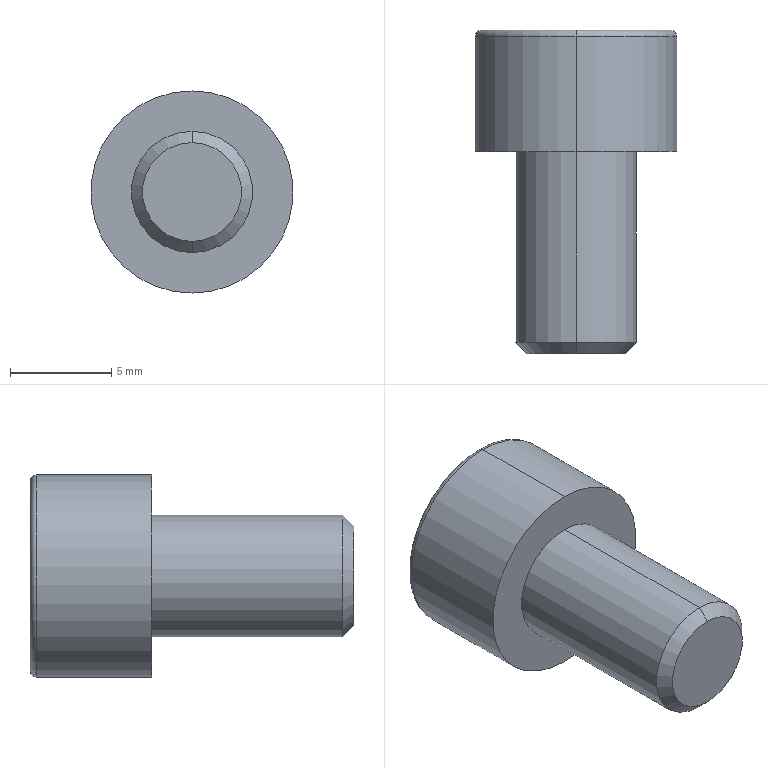Part | SolidWorks | features BaseBody 1 | 1 solid | 18 faces | box 10 x 16 x 10 mm | volume 683.613 mm3 | plane 10 | cylinder 4 | cone 2 | torus 2 | commonest cylinder face diameters 6 x2 10 x2
STEP:
#1=CARTESIAN_POINT('',(0.,-10.,-2.445));
#2=VERTEX_POINT('',#1);
#3=CARTESIAN_POINT('',(0.,-10.,2.445));
#4=VERTEX_POINT('',#3);
#5=CARTESIAN_POINT('',(0.,-10.,0.));
#6=DIRECTION('',(0.,-1.,0.));
#7=DIRECTION('',(0.,0.,-1.));
#8=AXIS2_PLACEMENT_3D('',#5,#6,#7);
#9=CIRCLE('',#8,2.445);
#10=EDGE_CURVE('',#2,#4,#9,.T.);
#11=ORIENTED_EDGE('',*,*,#10,.F.);
#12=CARTESIAN_POINT('',(0.,-9.445,-3.));
#13=VERTEX_POINT('',#12);
#14=CARTESIAN_POINT('',(0.,-10.,-2.445));
#15=DIRECTION('',(0.,0.7071,-0.7071));
#16=VECTOR('',#15,1000.);
#17=LINE('',#14,#16);
#18=EDGE_CURVE('',#2,#13,#17,.T.);
#19=ORIENTED_EDGE('',*,*,#18,.T.);
#20=CARTESIAN_POINT('',(0.,-9.445,3.));
#21=VERTEX_POINT('',#20);
#22=CARTESIAN_POINT('',(0.,-9.445,0.));
#23=DIRECTION('',(0.,1.,0.));
#24=DIRECTION('',(0.,0.,-1.));
#25=AXIS2_PLACEMENT_3D('',#22,#23,#24);
#26=CIRCLE('',#25,3.);
#27=EDGE_CURVE('',#21,#13,#26,.T.);
#28=ORIENTED_EDGE('',*,*,#27,.F.);
#29=CARTESIAN_POINT('',(0.,-10.,2.445));
#30=DIRECTION('',(0.,0.7071,0.7071));
#31=VECTOR('',#30,1000.);
#32=LINE('',#29,#31);
#33=EDGE_CURVE('',#4,#21,#32,.T.);
#34=ORIENTED_EDGE('',*,*,#33,.F.);
#35=EDGE_LOOP('',(#11,#19,#28,#34));
#36=FACE_OUTER_BOUND('',#35,.T.);
#37=CARTESIAN_POINT('',(0.,-10.,0.));
#38=DIRECTION('',(0.,1.,0.));
#39=DIRECTION('',(0.,0.,1.));
#40=AXIS2_PLACEMENT_3D('',#37,#38,#39);
#41=CONICAL_SURFACE('',#40,2.445,0.7854);
#42=ADVANCED_FACE('',(#36),#41,.T.);
#43=ORIENTED_EDGE('',*,*,#27,.T.);
#44=CARTESIAN_POINT('',(0.,0.,-3.));
#45=VERTEX_POINT('',#44);
#46=CARTESIAN_POINT('',(0.,-10.,-3.));
#47=DIRECTION('',(0.,1.,0.));
#48=VECTOR('',#47,1000.);
#49=LINE('',#46,#48);
#50=EDGE_CURVE('',#13,#45,#49,.T.);
#51=ORIENTED_EDGE('',*,*,#50,.T.);
#52=CARTESIAN_POINT('',(0.,0.,3.));
#53=VERTEX_POINT('',#52);
#54=CARTESIAN_POINT('',(0.,0.,0.));
#55=DIRECTION('',(0.,-1.,0.));
#56=DIRECTION('',(0.,0.,1.));
#57=AXIS2_PLACEMENT_3D('',#54,#55,#56);
#58=CIRCLE('',#57,3.);
#59=EDGE_CURVE('',#45,#53,#58,.T.);
#60=ORIENTED_EDGE('',*,*,#59,.T.);
#61=CARTESIAN_POINT('',(0.,-10.,3.));
#62=DIRECTION('',(0.,1.,0.));
#63=VECTOR('',#62,1000.);
#64=LINE('',#61,#63);
#65=EDGE_CURVE('',#21,#53,#64,.T.);
#66=ORIENTED_EDGE('',*,*,#65,.F.);
#67=EDGE_LOOP('',(#43,#51,#60,#66));
#68=FACE_OUTER_BOUND('',#67,.T.);
#69=CARTESIAN_POINT('',(0.,-10.,0.));
#70=DIRECTION('',(0.,1.,0.));
#71=DIRECTION('',(0.,0.,1.));
#72=AXIS2_PLACEMENT_3D('',#69,#70,#71);
#73=CYLINDRICAL_SURFACE('',#72,3.);
#74=ADVANCED_FACE('',(#68),#73,.T.);
#75=CARTESIAN_POINT('',(0.,5.7,-5.));
#76=VERTEX_POINT('',#75);
#77=CARTESIAN_POINT('',(0.,5.7,5.));
#78=VERTEX_POINT('',#77);
#79=CARTESIAN_POINT('',(0.,5.7,0.));
#80=DIRECTION('',(0.,-1.,0.));
#81=DIRECTION('',(0.,0.,1.));
#82=AXIS2_PLACEMENT_3D('',#79,#80,#81);
#83=CIRCLE('',#82,5.);
#84=EDGE_CURVE('',#76,#78,#83,.T.);
#85=ORIENTED_EDGE('',*,*,#84,.F.);
#86=CARTESIAN_POINT('',(0.,6.,-4.7));
#87=VERTEX_POINT('',#86);
#88=CARTESIAN_POINT('',(0.,5.7,-4.7));
#89=DIRECTION('',(1.,0.,0.));
#90=DIRECTION('',(0.,0.,-1.));
#91=AXIS2_PLACEMENT_3D('',#88,#89,#90);
#92=CIRCLE('',#91,0.3);
#93=EDGE_CURVE('',#76,#87,#92,.T.);
#94=ORIENTED_EDGE('',*,*,#93,.T.);
#95=CARTESIAN_POINT('',(0.,6.,4.7));
#96=VERTEX_POINT('',#95);
#97=CARTESIAN_POINT('',(0.,6.,0.));
#98=DIRECTION('',(0.,1.,0.));
#99=DIRECTION('',(0.,0.,1.));
#100=AXIS2_PLACEMENT_3D('',#97,#98,#99);
#101=CIRCLE('',#100,4.7);
#102=EDGE_CURVE('',#96,#87,#101,.T.);
#103=ORIENTED_EDGE('',*,*,#102,.F.);
#104=CARTESIAN_POINT('',(0.,5.7,4.7));
#105=DIRECTION('',(-1.,0.,0.));
#106=DIRECTION('',(0.,0.,1.));
#107=AXIS2_PLACEMENT_3D('',#104,#105,#106);
#108=CIRCLE('',#107,0.3);
#109=EDGE_CURVE('',#78,#96,#108,.T.);
#110=ORIENTED_EDGE('',*,*,#109,.F.);
#111=EDGE_LOOP('',(#85,#94,#103,#110));
#112=FACE_OUTER_BOUND('',#111,.T.);
#113=CARTESIAN_POINT('',(0.,5.7,0.));
#114=DIRECTION('',(0.,1.,0.));
#115=DIRECTION('',(0.,0.,1.));
#116=AXIS2_PLACEMENT_3D('',#113,#114,#115);
#117=TOROIDAL_SURFACE('',#116,4.7,0.3);
#118=ADVANCED_FACE('',(#112),#117,.T.);
#119=ORIENTED_EDGE('',*,*,#84,.T.);
#120=CARTESIAN_POINT('',(0.,0.,5.));
#121=VERTEX_POINT('',#120);
#122=CARTESIAN_POINT('',(0.,6.,5.));
#123=DIRECTION('',(0.,-1.,0.));
#124=VECTOR('',#123,1000.);
#125=LINE('',#122,#124);
#126=EDGE_CURVE('',#78,#121,#125,.T.);
#127=ORIENTED_EDGE('',*,*,#126,.T.);
#128=CARTESIAN_POINT('',(0.,0.,-5.));
#129=VERTEX_POINT('',#128);
#130=CARTESIAN_POINT('',(0.,0.,0.));
#131=DIRECTION('',(0.,1.,0.));
#132=DIRECTION('',(0.,0.,1.));
#133=AXIS2_PLACEMENT_3D('',#130,#131,#132);
#134=CIRCLE('',#133,5.);
#135=EDGE_CURVE('',#121,#129,#134,.T.);
#136=ORIENTED_EDGE('',*,*,#135,.T.);
#137=CARTESIAN_POINT('',(0.,6.,-5.));
#138=DIRECTION('',(0.,-1.,0.));
#139=VECTOR('',#138,1000.);
#140=LINE('',#137,#139);
#141=EDGE_CURVE('',#76,#129,#140,.T.);
#142=ORIENTED_EDGE('',*,*,#141,.F.);
#143=EDGE_LOOP('',(#119,#127,#136,#142));
#144=FACE_OUTER_BOUND('',#143,.T.);
#145=CARTESIAN_POINT('',(0.,6.,0.));
#146=DIRECTION('',(0.,-1.,0.));
#147=DIRECTION('',(0.,0.,-1.));
#148=AXIS2_PLACEMENT_3D('',#145,#146,#147);
#149=CYLINDRICAL_SURFACE('',#148,5.);
#150=ADVANCED_FACE('',(#144),#149,.T.);
#151=CARTESIAN_POINT('',(0.,-10.,0.));
#152=DIRECTION('',(0.,-1.,0.));
#153=DIRECTION('',(0.,0.,-1.));
#154=AXIS2_PLACEMENT_3D('',#151,#152,#153);
#155=CIRCLE('',#154,2.445);
#156=EDGE_CURVE('',#4,#2,#155,.T.);
#157=ORIENTED_EDGE('',*,*,#156,.T.);
#158=ORIENTED_EDGE('',*,*,#10,.T.);
#159=EDGE_LOOP('',(#157,#158));
#160=FACE_OUTER_BOUND('',#159,.T.);
#161=CARTESIAN_POINT('',(0.,-10.,0.));
#162=DIRECTION('',(0.,-1.,0.));
#163=DIRECTION('',(0.,0.,-1.));
#164=AXIS2_PLACEMENT_3D('',#161,#162,#163);
#165=PLANE('',#164);
#166=ADVANCED_FACE('',(#160),#165,.T.);
#167=CARTESIAN_POINT('',(1.466,3.,2.54));
#168=VERTEX_POINT('',#167);
#169=CARTESIAN_POINT('',(2.933,3.,0.));
#170=VERTEX_POINT('',#169);
#171=CARTESIAN_POINT('',(1.466,3.,2.54));
#172=DIRECTION('',(0.5,0.,-0.866));
#173=VECTOR('',#172,1000.);
#174=LINE('',#171,#173);
#175=EDGE_CURVE('',#168,#170,#174,.T.);
#176=ORIENTED_EDGE('',*,*,#175,.T.);
#177=CARTESIAN_POINT('',(1.466,3.,-2.54));
#178=VERTEX_POINT('',#177);
#179=CARTESIAN_POINT('',(2.933,3.,0.));
#180=DIRECTION('',(-0.5,0.,-0.866));
#181=VECTOR('',#180,1000.);
#182=LINE('',#179,#181);
#183=EDGE_CURVE('',#170,#178,#182,.T.);
#184=ORIENTED_EDGE('',*,*,#183,.T.);
#185=CARTESIAN_POINT('',(-1.466,3.,-2.54));
#186=VERTEX_POINT('',#185);
#187=CARTESIAN_POINT('',(1.466,3.,-2.54));
#188=DIRECTION('',(-1.,0.,0.));
#189=VECTOR('',#188,1000.);
#190=LINE('',#187,#189);
#191=EDGE_CURVE('',#178,#186,#190,.T.);
#192=ORIENTED_EDGE('',*,*,#191,.T.);
#193=CARTESIAN_POINT('',(-2.933,3.,0.));
#194=VERTEX_POINT('',#193);
#195=CARTESIAN_POINT('',(-1.466,3.,-2.54));
#196=DIRECTION('',(-0.5,0.,0.866));
#197=VECTOR('',#196,1000.);
#198=LINE('',#195,#197);
#199=EDGE_CURVE('',#186,#194,#198,.T.);
#200=ORIENTED_EDGE('',*,*,#199,.T.);
#201=CARTESIAN_POINT('',(-1.466,3.,2.54));
#202=VERTEX_POINT('',#201);
#203=CARTESIAN_POINT('',(-2.933,3.,0.));
#204=DIRECTION('',(0.5,0.,0.866));
#205=VECTOR('',#204,1000.);
#206=LINE('',#203,#205);
#207=EDGE_CURVE('',#194,#202,#206,.T.);
#208=ORIENTED_EDGE('',*,*,#207,.T.);
#209=CARTESIAN_POINT('',(-1.466,3.,2.54));
#210=DIRECTION('',(1.,0.,0.));
#211=VECTOR('',#210,1000.);
#212=LINE('',#209,#211);
#213=EDGE_CURVE('',#202,#168,#212,.T.);
#214=ORIENTED_EDGE('',*,*,#213,.T.);
#215=EDGE_LOOP('',(#176,#184,#192,#200,#208,#214));
#216=FACE_OUTER_BOUND('',#215,.T.);
#217=CARTESIAN_POINT('',(0.,3.,0.));
#218=DIRECTION('',(0.,1.,0.));
#219=DIRECTION('',(1.,0.,0.));
#220=AXIS2_PLACEMENT_3D('',#217,#218,#219);
#221=PLANE('',#220);
#222=ADVANCED_FACE('',(#216),#221,.T.);
#223=CARTESIAN_POINT('',(2.933,6.,0.));
#224=VERTEX_POINT('',#223);
#225=CARTESIAN_POINT('',(1.466,6.,-2.54));
#226=VERTEX_POINT('',#225);
#227=CARTESIAN_POINT('',(2.933,6.,0.));
#228=DIRECTION('',(-0.5,0.,-0.866));
#229=VECTOR('',#228,1000.);
#230=LINE('',#227,#229);
#231=EDGE_CURVE('',#224,#226,#230,.T.);
#232=ORIENTED_EDGE('',*,*,#231,.T.);
#233=CARTESIAN_POINT('',(1.466,3.,-2.54));
#234=DIRECTION('',(0.,1.,0.));
#235=VECTOR('',#234,1000.);
#236=LINE('',#233,#235);
#237=EDGE_CURVE('',#178,#226,#236,.T.);
#238=ORIENTED_EDGE('',*,*,#237,.F.);
#239=ORIENTED_EDGE('',*,*,#183,.F.);
#240=CARTESIAN_POINT('',(2.933,3.,0.));
#241=DIRECTION('',(0.,1.,0.));
#242=VECTOR('',#241,1000.);
#243=LINE('',#240,#242);
#244=EDGE_CURVE('',#170,#224,#243,.T.);
#245=ORIENTED_EDGE('',*,*,#244,.T.);
#246=EDGE_LOOP('',(#232,#238,#239,#245));
#247=FACE_OUTER_BOUND('',#246,.T.);
#248=CARTESIAN_POINT('',(2.933,3.,0.));
#249=DIRECTION('',(0.866,0.,-0.5));
#250=DIRECTION('',(0.,-1.,0.));
#251=AXIS2_PLACEMENT_3D('',#248,#249,#250);
#252=PLANE('',#251);
#253=ADVANCED_FACE('',(#247),#252,.F.);
#254=CARTESIAN_POINT('',(-1.466,6.,-2.54));
#255=VERTEX_POINT('',#254);
#256=CARTESIAN_POINT('',(1.466,6.,-2.54));
#257=DIRECTION('',(-1.,0.,0.));
#258=VECTOR('',#257,1000.);
#259=LINE('',#256,#258);
#260=EDGE_CURVE('',#226,#255,#259,.T.);
#261=ORIENTED_EDGE('',*,*,#260,.T.);
#262=CARTESIAN_POINT('',(-1.466,3.,-2.54));
#263=DIRECTION('',(0.,1.,0.));
#264=VECTOR('',#263,1000.);
#265=LINE('',#262,#264);
#266=EDGE_CURVE('',#186,#255,#265,.T.);
#267=ORIENTED_EDGE('',*,*,#266,.F.);
#268=ORIENTED_EDGE('',*,*,#191,.F.);
#269=ORIENTED_EDGE('',*,*,#237,.T.);
#270=EDGE_LOOP('',(#261,#267,#268,#269));
#271=FACE_OUTER_BOUND('',#270,.T.);
#272=CARTESIAN_POINT('',(1.466,3.,-2.54));
#273=DIRECTION('',(0.,0.,-1.));
#274=DIRECTION('',(0.,-1.,0.));
#275=AXIS2_PLACEMENT_3D('',#272,#273,#274);
#276=PLANE('',#275);
#277=ADVANCED_FACE('',(#271),#276,.F.);
#278=CARTESIAN_POINT('',(-2.933,6.,0.));
#279=VERTEX_POINT('',#278);
#280=CARTESIAN_POINT('',(-1.466,6.,-2.54));
#281=DIRECTION('',(-0.5,0.,0.866));
#282=VECTOR('',#281,1000.);
#283=LINE('',#280,#282);
#284=EDGE_CURVE('',#255,#279,#283,.T.);
#285=ORIENTED_EDGE('',*,*,#284,.T.);
#286=CARTESIAN_POINT('',(-2.933,3.,0.));
#287=DIRECTION('',(0.,1.,0.));
#288=VECTOR('',#287,1000.);
#289=LINE('',#286,#288);
#290=EDGE_CURVE('',#194,#279,#289,.T.);
#291=ORIENTED_EDGE('',*,*,#290,.F.);
#292=ORIENTED_EDGE('',*,*,#199,.F.);
#293=ORIENTED_EDGE('',*,*,#266,.T.);
#294=EDGE_LOOP('',(#285,#291,#292,#293));
#295=FACE_OUTER_BOUND('',#294,.T.);
#296=CARTESIAN_POINT('',(-1.466,3.,-2.54));
#297=DIRECTION('',(-0.866,0.,-0.5));
#298=DIRECTION('',(-0.5,0.,0.866));
#299=AXIS2_PLACEMENT_3D('',#296,#297,#298);
#300=PLANE('',#299);
#301=ADVANCED_FACE('',(#295),#300,.F.);
#302=CARTESIAN_POINT('',(-1.466,6.,2.54));
#303=VERTEX_POINT('',#302);
#304=CARTESIAN_POINT('',(-2.933,6.,0.));
#305=DIRECTION('',(0.5,0.,0.866));
#306=VECTOR('',#305,1000.);
#307=LINE('',#304,#306);
#308=EDGE_CURVE('',#279,#303,#307,.T.);
#309=ORIENTED_EDGE('',*,*,#308,.T.);
#310=CARTESIAN_POINT('',(-1.466,3.,2.54));
#311=DIRECTION('',(0.,1.,0.));
#312=VECTOR('',#311,1000.);
#313=LINE('',#310,#312);
#314=EDGE_CURVE('',#202,#303,#313,.T.);
#315=ORIENTED_EDGE('',*,*,#314,.F.);
#316=ORIENTED_EDGE('',*,*,#207,.F.);
#317=ORIENTED_EDGE('',*,*,#290,.T.);
#318=EDGE_LOOP('',(#309,#315,#316,#317));
#319=FACE_OUTER_BOUND('',#318,.T.);
#320=CARTESIAN_POINT('',(-2.933,3.,0.));
#321=DIRECTION('',(-0.866,0.,0.5));
#322=DIRECTION('',(0.,1.,0.));
#323=AXIS2_PLACEMENT_3D('',#320,#321,#322);
#324=PLANE('',#323);
#325=ADVANCED_FACE('',(#319),#324,.F.);
#326=CARTESIAN_POINT('',(1.466,6.,2.54));
#327=VERTEX_POINT('',#326);
#328=CARTESIAN_POINT('',(-1.466,6.,2.54));
#329=DIRECTION('',(1.,0.,0.));
#330=VECTOR('',#329,1000.);
#331=LINE('',#328,#330);
#332=EDGE_CURVE('',#303,#327,#331,.T.);
#333=ORIENTED_EDGE('',*,*,#332,.T.);
#334=CARTESIAN_POINT('',(1.466,3.,2.54));
#335=DIRECTION('',(0.,1.,0.));
#336=VECTOR('',#335,1000.);
#337=LINE('',#334,#336);
#338=EDGE_CURVE('',#168,#327,#337,.T.);
#339=ORIENTED_EDGE('',*,*,#338,.F.);
#340=ORIENTED_EDGE('',*,*,#213,.F.);
#341=ORIENTED_EDGE('',*,*,#314,.T.);
#342=EDGE_LOOP('',(#333,#339,#340,#341));
#343=FACE_OUTER_BOUND('',#342,.T.);
#344=CARTESIAN_POINT('',(-1.466,3.,2.54));
#345=DIRECTION('',(0.,0.,1.));
#346=DIRECTION('',(1.,0.,0.));
#347=AXIS2_PLACEMENT_3D('',#344,#345,#346);
#348=PLANE('',#347);
#349=ADVANCED_FACE('',(#343),#348,.F.);
#350=CARTESIAN_POINT('',(1.466,6.,2.54));
#351=DIRECTION('',(0.5,0.,-0.866));
#352=VECTOR('',#351,1000.);
#353=LINE('',#350,#352);
#354=EDGE_CURVE('',#327,#224,#353,.T.);
#355=ORIENTED_EDGE('',*,*,#354,.T.);
#356=ORIENTED_EDGE('',*,*,#244,.F.);
#357=ORIENTED_EDGE('',*,*,#175,.F.);
#358=ORIENTED_EDGE('',*,*,#338,.T.);
#359=EDGE_LOOP('',(#355,#356,#357,#358));
#360=FACE_OUTER_BOUND('',#359,.T.);
#361=CARTESIAN_POINT('',(1.466,3.,2.54));
#362=DIRECTION('',(0.866,0.,0.5));
#363=DIRECTION('',(0.,-1.,0.));
#364=AXIS2_PLACEMENT_3D('',#361,#362,#363);
#365=PLANE('',#364);
#366=ADVANCED_FACE('',(#360),#365,.F.);
#367=ORIENTED_EDGE('',*,*,#354,.F.);
#368=ORIENTED_EDGE('',*,*,#332,.F.);
#369=ORIENTED_EDGE('',*,*,#308,.F.);
#370=ORIENTED_EDGE('',*,*,#284,.F.);
#371=ORIENTED_EDGE('',*,*,#260,.F.);
#372=ORIENTED_EDGE('',*,*,#231,.F.);
#373=EDGE_LOOP('',(#367,#368,#369,#370,#371,#372));
#374=FACE_BOUND('',#373,.T.);
#375=ORIENTED_EDGE('',*,*,#102,.T.);
#376=CARTESIAN_POINT('',(0.,6.,0.));
#377=DIRECTION('',(0.,1.,0.));
#378=DIRECTION('',(0.,0.,1.));
#379=AXIS2_PLACEMENT_3D('',#376,#377,#378);
#380=CIRCLE('',#379,4.7);
#381=EDGE_CURVE('',#87,#96,#380,.T.);
#382=ORIENTED_EDGE('',*,*,#381,.T.);
#383=EDGE_LOOP('',(#375,#382));
#384=FACE_OUTER_BOUND('',#383,.T.);
#385=CARTESIAN_POINT('',(0.,6.,0.));
#386=DIRECTION('',(0.,1.,0.));
#387=DIRECTION('',(1.,0.,0.));
#388=AXIS2_PLACEMENT_3D('',#385,#386,#387);
#389=PLANE('',#388);
#390=ADVANCED_FACE('',(#374,#384),#389,.T.);
#391=CARTESIAN_POINT('',(0.,0.,0.));
#392=DIRECTION('',(0.,-1.,0.));
#393=DIRECTION('',(0.,0.,1.));
#394=AXIS2_PLACEMENT_3D('',#391,#392,#393);
#395=CIRCLE('',#394,3.);
#396=EDGE_CURVE('',#53,#45,#395,.T.);
#397=ORIENTED_EDGE('',*,*,#396,.F.);
#398=ORIENTED_EDGE('',*,*,#59,.F.);
#399=EDGE_LOOP('',(#397,#398));
#400=FACE_BOUND('',#399,.T.);
#401=CARTESIAN_POINT('',(0.,0.,0.));
#402=DIRECTION('',(0.,1.,0.));
#403=DIRECTION('',(0.,0.,1.));
#404=AXIS2_PLACEMENT_3D('',#401,#402,#403);
#405=CIRCLE('',#404,5.);
#406=EDGE_CURVE('',#129,#121,#405,.T.);
#407=ORIENTED_EDGE('',*,*,#406,.F.);
#408=ORIENTED_EDGE('',*,*,#135,.F.);
#409=EDGE_LOOP('',(#407,#408));
#410=FACE_OUTER_BOUND('',#409,.T.);
#411=CARTESIAN_POINT('',(0.,0.,0.));
#412=DIRECTION('',(0.,1.,0.));
#413=DIRECTION('',(1.,0.,0.));
#414=AXIS2_PLACEMENT_3D('',#411,#412,#413);
#415=PLANE('',#414);
#416=ADVANCED_FACE('',(#400,#410),#415,.F.);
#417=ORIENTED_EDGE('',*,*,#126,.F.);
#418=CARTESIAN_POINT('',(0.,5.7,0.));
#419=DIRECTION('',(0.,-1.,0.));
#420=DIRECTION('',(0.,0.,1.));
#421=AXIS2_PLACEMENT_3D('',#418,#419,#420);
#422=CIRCLE('',#421,5.);
#423=EDGE_CURVE('',#78,#76,#422,.T.);
#424=ORIENTED_EDGE('',*,*,#423,.T.);
#425=ORIENTED_EDGE('',*,*,#141,.T.);
#426=ORIENTED_EDGE('',*,*,#406,.T.);
#427=EDGE_LOOP('',(#417,#424,#425,#426));
#428=FACE_OUTER_BOUND('',#427,.T.);
#429=CARTESIAN_POINT('',(0.,6.,0.));
#430=DIRECTION('',(0.,-1.,0.));
#431=DIRECTION('',(0.,0.,-1.));
#432=AXIS2_PLACEMENT_3D('',#429,#430,#431);
#433=CYLINDRICAL_SURFACE('',#432,5.);
#434=ADVANCED_FACE('',(#428),#433,.T.);
#435=ORIENTED_EDGE('',*,*,#93,.F.);
#436=ORIENTED_EDGE('',*,*,#423,.F.);
#437=ORIENTED_EDGE('',*,*,#109,.T.);
#438=ORIENTED_EDGE('',*,*,#381,.F.);
#439=EDGE_LOOP('',(#435,#436,#437,#438));
#440=FACE_OUTER_BOUND('',#439,.T.);
#441=CARTESIAN_POINT('',(0.,5.7,0.));
#442=DIRECTION('',(0.,1.,0.));
#443=DIRECTION('',(0.,0.,1.));
#444=AXIS2_PLACEMENT_3D('',#441,#442,#443);
#445=TOROIDAL_SURFACE('',#444,4.7,0.3);
#446=ADVANCED_FACE('',(#440),#445,.T.);
#447=ORIENTED_EDGE('',*,*,#50,.F.);
#448=CARTESIAN_POINT('',(0.,-9.445,0.));
#449=DIRECTION('',(0.,1.,0.));
#450=DIRECTION('',(0.,0.,-1.));
#451=AXIS2_PLACEMENT_3D('',#448,#449,#450);
#452=CIRCLE('',#451,3.);
#453=EDGE_CURVE('',#13,#21,#452,.T.);
#454=ORIENTED_EDGE('',*,*,#453,.T.);
#455=ORIENTED_EDGE('',*,*,#65,.T.);
#456=ORIENTED_EDGE('',*,*,#396,.T.);
#457=EDGE_LOOP('',(#447,#454,#455,#456));
#458=FACE_OUTER_BOUND('',#457,.T.);
#459=CARTESIAN_POINT('',(0.,-10.,0.));
#460=DIRECTION('',(0.,1.,0.));
#461=DIRECTION('',(0.,0.,1.));
#462=AXIS2_PLACEMENT_3D('',#459,#460,#461);
#463=CYLINDRICAL_SURFACE('',#462,3.);
#464=ADVANCED_FACE('',(#458),#463,.T.);
#465=ORIENTED_EDGE('',*,*,#18,.F.);
#466=ORIENTED_EDGE('',*,*,#156,.F.);
#467=ORIENTED_EDGE('',*,*,#33,.T.);
#468=ORIENTED_EDGE('',*,*,#453,.F.);
#469=EDGE_LOOP('',(#465,#466,#467,#468));
#470=FACE_OUTER_BOUND('',#469,.T.);
#471=CARTESIAN_POINT('',(0.,-10.,0.));
#472=DIRECTION('',(0.,1.,0.));
#473=DIRECTION('',(0.,0.,1.));
#474=AXIS2_PLACEMENT_3D('',#471,#472,#473);
#475=CONICAL_SURFACE('',#474,2.445,0.7854);
#476=ADVANCED_FACE('',(#470),#475,.T.);
#477=CLOSED_SHELL('',(#42,#74,#118,#150,#166,#222,#253,#277,#301,#325,#349,#366,#390,#416,#434,#446,#464,#476));
#478=MANIFOLD_SOLID_BREP('',#477);
#479=CARTESIAN_POINT('',(0.,0.,0.));
#480=DIRECTION('',(0.,0.,1.));
#481=DIRECTION('',(1.,0.,0.));
#482=AXIS2_PLACEMENT_3D('',#479,#480,#481);
#483=(LENGTH_UNIT()NAMED_UNIT(*)SI_UNIT(.MILLI.,.METRE.));
#484=UNCERTAINTY_MEASURE_WITH_UNIT(LENGTH_MEASURE(0.00001),#483,'','');
#485=(NAMED_UNIT(*)PLANE_ANGLE_UNIT()SI_UNIT($,.RADIAN.));
#486=(NAMED_UNIT(*)SI_UNIT($,.STERADIAN.)SOLID_ANGLE_UNIT());
#487=(GEOMETRIC_REPRESENTATION_CONTEXT(3)GLOBAL_UNCERTAINTY_ASSIGNED_CONTEXT((#484))GLOBAL_UNIT_ASSIGNED_CONTEXT((#483,#485,#486))REPRESENTATION_CONTEXT('',''));
#488=ADVANCED_BREP_SHAPE_REPRESENTATION('',(#478,#482),#487);